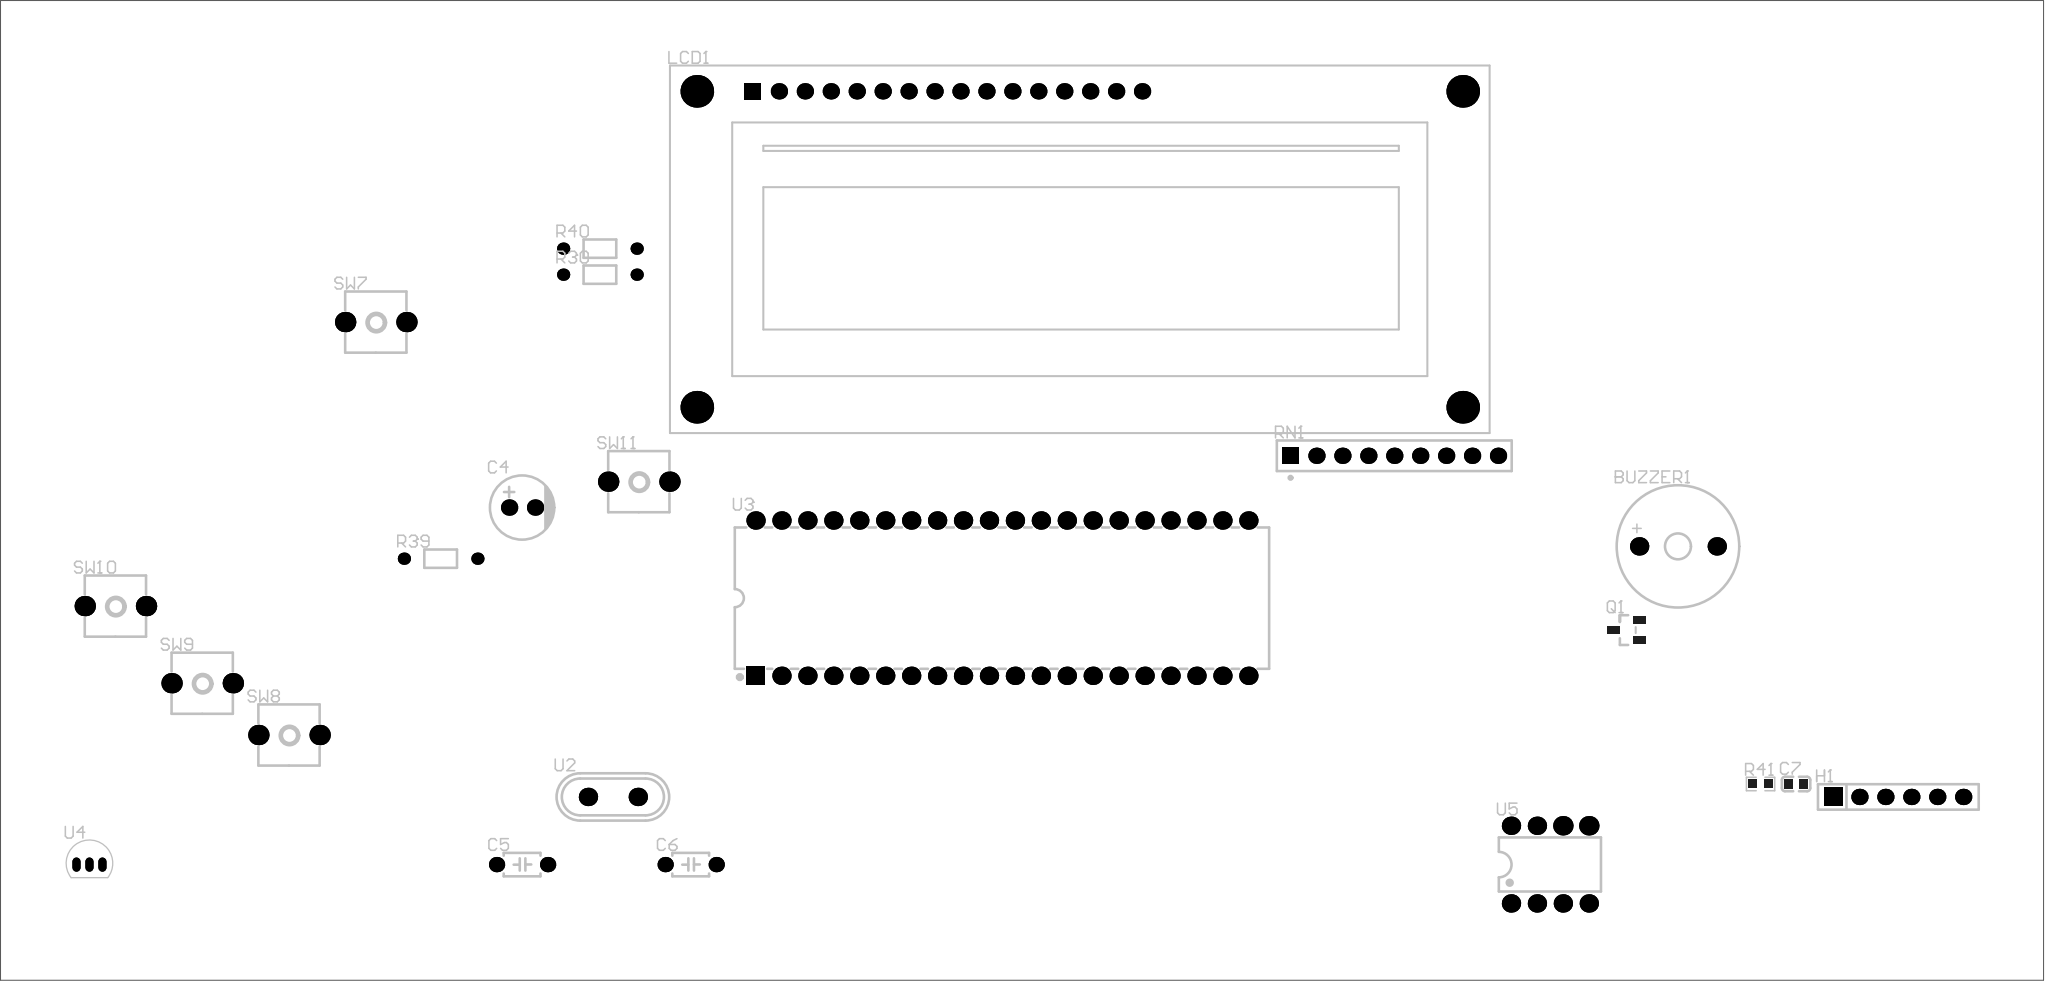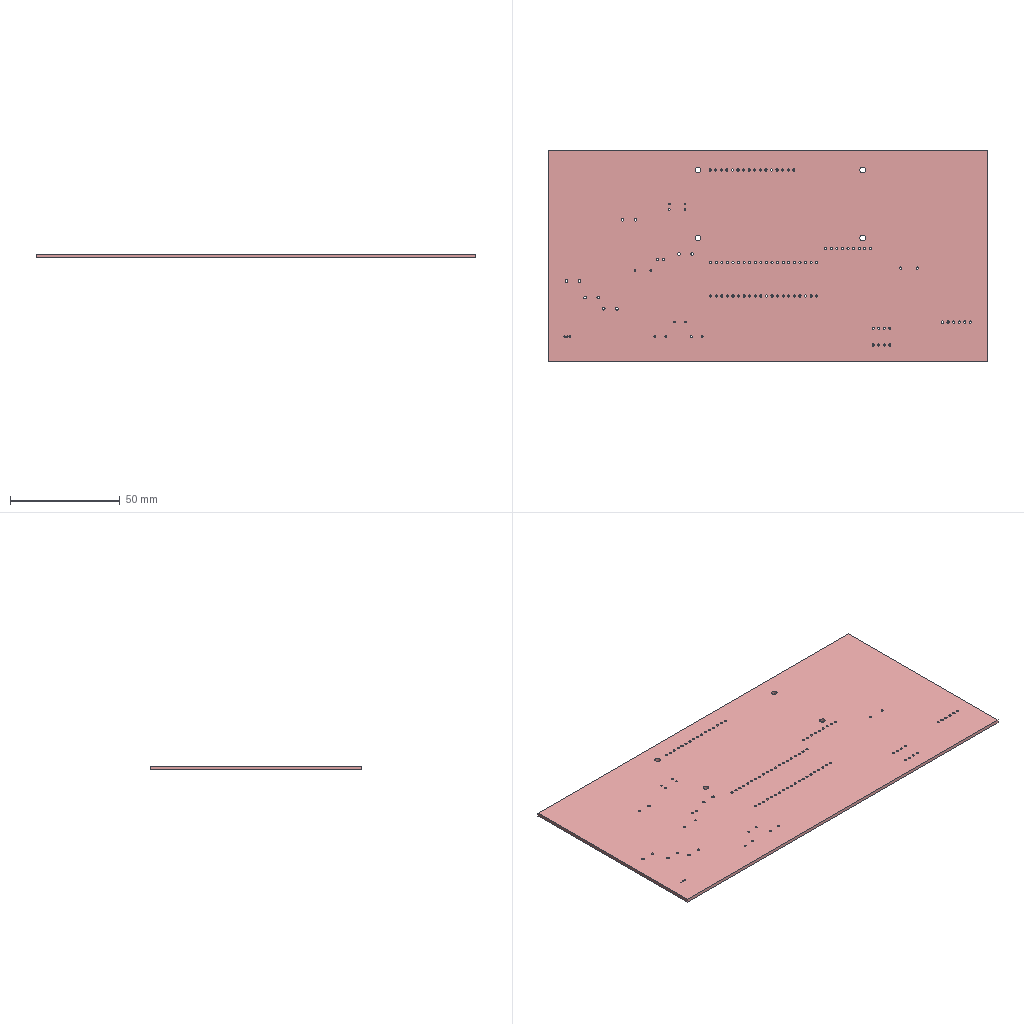Circuit board layout | Altium Designer | box 200.1 x 96.1 x 1.6 mm
Layer stack:
# Altium Designer layer stack of  (unit mm; dielectric type: 0 none, 1 core, 2 prepreg, 3 surface material)
index,name,kind,layer,copper_thickness_mm,dielectric_type,dielectric_thickness_mm,dielectric_material,dielectric_constant
0,Top Paste Mask Layer,other,,,,,,
1,Top Silkscreen Layer,other,,,,,,
2,Top Solder Mask Layer,dielectric,,,3,0.01,,3.3
3,Top Layer,copper,Top Layer,0.035,,,,
4,Dielectric1,dielectric,,,3,1.51,FR4,4.5
5,Bottom Layer,copper,Bottom Layer,0.035,,,,
6,Bottom Solder Mask Layer,dielectric,,,3,0.01,,3.3
7,Bottom Silkscreen Layer,other,,,,,,
8,Bottom Paste Mask Layer,other,,,,,,
# drill layer pairs: low layer,high layer
drill_pair,Top Layer,Bottom Layer
Part placement:
Designator,Comment,Layer,Footprint,Center-X(mm),Center-Y(mm),Rotation
BUZZER1,buzzer-12X9,TopLayer,BUZ-TH_BD12.0-P7.60-D0.6-FD,234.111,112.425,0
C4,10uF,TopLayer,CAP-TH_BD6.3-P2.50-D1.0-FD,120.925,116.235,0
C5,30pF,TopLayer,CAP-TH_L3.6-W2.3-P5.00-D0.5,120.925,81.199,0
C6,30pF,TopLayer,CAP-TH_L3.6-W2.3-P5.00-D0.5,137.435,81.199,0
C7,22pF,TopLayer,C0603,245.677,89.109,0
H1,,TopLayer,HDR-TH_6P-P2.54-V-F,255.691,87.838,0
LCD1,LMB162ADC,TopLayer,LCD1602,175.535,141.576,0
Q1,,TopLayer,S8550P_SOT,229.073,104.21,0
R30,1kΩ,TopLayer,Res_1/8W,128.545,139.087,0
R39,10kΩ,TopLayer,Res_1/8W,112.95,111.218,0
R40,10kΩ,TopLayer,Res_1/8W,128.545,141.639,0
R41,51K,TopLayer,R0603,242.199,89.109,0
RN1,-,TopLayer,RES-ARRAY-TH_9P-P2.54-D1.0,206.331,121.315,0
SW7,Tact switch, 6*6*5 plastic head, 260G, travel 0.25mm, through-hole, middle 2 pins,TopLayer,KEY-TH_2P-L6.0-W6.0-P5.00,106.6,134.433,0
SW8,Tact switch, 6*6*5 plastic head, 260G, travel 0.25mm, through-hole, middle 2 pins,TopLayer,KEY-TH_2P-L6.0-W6.0-P5.00,98.1,93.916,0
SW9,Tact switch, 6*6*5 plastic head, 260G, travel 0.25mm, through-hole, middle 2 pins,TopLayer,KEY-TH_2P-L6.0-W6.0-P5.00,89.6,98.996,0
SW10,Tact switch, 6*6*5 plastic head, 260G, travel 0.25mm, through-hole, middle 2 pins,TopLayer,KEY-TH_2P-L6.0-W6.0-P5.00,81.1,106.565,0
SW11,Tact switch, 6*6*5 plastic head, 260G, travel 0.25mm, through-hole, middle 2 pins,TopLayer,KEY-TH_2P-L6.0-W6.0-P5.00,132.355,118.775,0
U2,12MHz,TopLayer,HC-49US_L11.0-W4.6-P4.88,129.815,87.838,0
U3,STC89C516RD+40I-PDIP40,TopLayer,DIP-40_L52.3-W13.9-P2.54-LS15.2-BL,167.915,107.345,0
U4,DS18B20,TopLayer,TO-92-3_L4.6-W3.6-P1.27-L-1,78.56,81.199,0
U5,ADC0832BCN,TopLayer,PDIP-8_L9.6-W6.4-P2.54-LS7.6-BL,221.571,81.199,0
Pad and via stacks:
# Altium Designer via and pad stacks of  (unit mm). Each distinct definition once, with the count of objects using it.
# via: kind,start_layer,end_layer,hole_mm,diameter_mm,mode(0 simple;1 top-mid-bottom;2 full stack),diameter_per_layer,count,example_net
# pad: kind,layer,hole_mm,hole_type(0 round;1 square;2 slot),plating,top_size,top_shape(1 round;2 rect;3 octagon;9 rounded rect),mid_size,bottom_size,mode,footprint,size_per_layer,count,example
pad,Multi-Layer,1,0,plated,1.8x1.8,1,1.8x1.8,1.8x1.8,0,BUZ-TH_BD12.0-P7.60-D0.6-FD,,2,BUZZER1.2
pad,Multi-Layer,1,0,plated,1.6x1.6,1,1.6x1.6,1.6x1.6,0,CAP-TH_BD6.3-P2.50-D1.0-FD,,2,C4.1
pad,Multi-Layer,0.9,0,plated,1.5x1.5,1,1.5x1.5,1.5x1.5,0,CAP-TH_L3.6-W2.3-P5.00-D0.5,,4,C5.1
pad,Multi-Layer,1.02,0,plated,1.6x1.6,1,1.6x1.6,1.6x1.6,0,HDR-TH_6P-P2.54-V-F,,5,H1.6
pad,Multi-Layer,1.02,0,plated,1.8x1.8,2,1.8x1.8,1.8x1.8,0,HDR-TH_6P-P2.54-V-F,,1,H1.1
pad,Multi-Layer,1,0,plated,1.6x1.6,1,1.6x1.6,1.6x1.6,0,LCD1602,,15,LCD1.16
pad,Multi-Layer,1,0,plated,1.6x1.6,2,1.6x1.6,1.6x1.6,0,LCD1602,,1,LCD1.1
pad,Multi-Layer,2.5,2,plated,3.2x3.2,1,3.2x3.2,3.2x3.2,0,LCD1602,,4,LCD1.0
pad,Multi-Layer,0.8001,0,plated,1.199x1.199,1,1.199x1.199,1.199x1.199,0,Res_1/8W,,6,R30.1
pad,Multi-Layer,1,0,plated,1.6x1.6,2,1.6x1.6,1.6x1.6,0,RES-ARRAY-TH_9P-P2.54-D1.0,,1,RN1.1
pad,Multi-Layer,1,0,plated,1.6x1.6,1,1.6x1.6,1.6x1.6,0,RES-ARRAY-TH_9P-P2.54-D1.0,,8,RN1.2
pad,Multi-Layer,1.2,0,plated,2x2,1,2x2,2x2,0,KEY-TH_2P-L6.0-W6.0-P5.00,,10,SW7.2
pad,Multi-Layer,0.8,0,plated,1.8x1.8,1,1.8x1.8,1.8x1.8,0,HC-49US_L11.0-W4.6-P4.88,,2,U2.1
pad,Multi-Layer,1,0,plated,1.8x1.8,1,1.8x1.8,1.8x1.8,0,DIP-40_L52.3-W13.9-P2.54-LS15.2-BL,,39,U3.19
pad,Multi-Layer,1,0,plated,1.8x1.8,2,1.8x1.8,1.8x1.8,0,DIP-40_L52.3-W13.9-P2.54-LS15.2-BL,,1,U3.1
pad,Multi-Layer,0.6,2,plated,0.8x1.4,1,0.8x1.4,0.8x1.4,0,TO-92-3_L4.6-W3.6-P1.27-L-1,,3,U4.3
pad,Multi-Layer,1,0,plated,1.8x1.8,1,1.8x1.8,1.8x1.8,0,PDIP-8_L9.6-W6.4-P2.54-LS7.6-BL,,6,U5.1
pad,Multi-Layer,1,0,plated,1.905x1.905,1,1.905x1.905,1.905x1.905,0,PDIP-8_L9.6-W6.4-P2.54-LS7.6-BL,,2,U5.5
pad,Top Layer,0,0,plated,0.8x0.9,2,0.8x0.9,0.8x0.9,0,C0603,,2,C7.2
pad,Top Layer,0,0,plated,0.701x1.25,2,0.701x1.25,0.701x1.25,0,S8550P_SOT,,3,Q1.3
pad,Top Layer,0,0,plated,0.8065x0.864,2,0.8065x0.864,0.8065x0.864,0,R0603,,2,R41.2